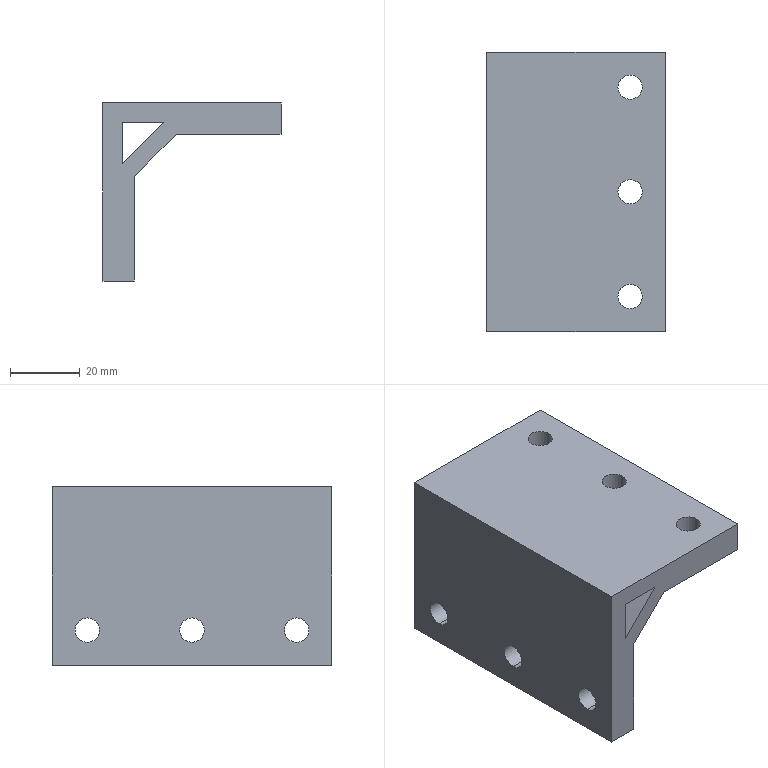Part | SolidWorks | features BaseBody 1 | 1 solid | 24 faces | box 51 x 80 x 51 mm | volume 64882 mm3 | cylinder 12 | plane 12 | commonest cylinder face diameters 7 x12
STEP:
#1=CARTESIAN_POINT('',(44.5,-30.,0.));
#2=VERTEX_POINT('',#1);
#3=CARTESIAN_POINT('',(37.5,-30.,0.));
#4=VERTEX_POINT('',#3);
#5=CARTESIAN_POINT('',(41.,-30.,0.));
#6=DIRECTION('',(0.,0.,-1.));
#7=DIRECTION('',(1.,0.,0.));
#8=AXIS2_PLACEMENT_3D('',#5,#6,#7);
#9=CIRCLE('',#8,3.5);
#10=EDGE_CURVE('',#2,#4,#9,.T.);
#11=ORIENTED_EDGE('',*,*,#10,.F.);
#12=CARTESIAN_POINT('',(44.5,-30.,-9.));
#13=VERTEX_POINT('',#12);
#14=CARTESIAN_POINT('',(44.5,-30.,0.));
#15=DIRECTION('',(0.,0.,-1.));
#16=VECTOR('',#15,1000.);
#17=LINE('',#14,#16);
#18=EDGE_CURVE('',#2,#13,#17,.T.);
#19=ORIENTED_EDGE('',*,*,#18,.T.);
#20=CARTESIAN_POINT('',(37.5,-30.,-9.));
#21=VERTEX_POINT('',#20);
#22=CARTESIAN_POINT('',(41.,-30.,-9.));
#23=DIRECTION('',(0.,0.,-1.));
#24=DIRECTION('',(1.,0.,0.));
#25=AXIS2_PLACEMENT_3D('',#22,#23,#24);
#26=CIRCLE('',#25,3.5);
#27=EDGE_CURVE('',#13,#21,#26,.T.);
#28=ORIENTED_EDGE('',*,*,#27,.T.);
#29=CARTESIAN_POINT('',(37.5,-30.,0.));
#30=DIRECTION('',(0.,0.,-1.));
#31=VECTOR('',#30,1000.);
#32=LINE('',#29,#31);
#33=EDGE_CURVE('',#4,#21,#32,.T.);
#34=ORIENTED_EDGE('',*,*,#33,.F.);
#35=EDGE_LOOP('',(#11,#19,#28,#34));
#36=FACE_OUTER_BOUND('',#35,.T.);
#37=CARTESIAN_POINT('',(41.,-30.,0.));
#38=DIRECTION('',(0.,0.,-1.));
#39=DIRECTION('',(-1.,0.,0.));
#40=AXIS2_PLACEMENT_3D('',#37,#38,#39);
#41=CYLINDRICAL_SURFACE('',#40,3.5);
#42=ADVANCED_FACE('',(#36),#41,.F.);
#43=CARTESIAN_POINT('',(44.5,0.,0.));
#44=VERTEX_POINT('',#43);
#45=CARTESIAN_POINT('',(37.5,0.,0.));
#46=VERTEX_POINT('',#45);
#47=CARTESIAN_POINT('',(41.,0.,0.));
#48=DIRECTION('',(0.,0.,-1.));
#49=DIRECTION('',(-1.,0.,0.));
#50=AXIS2_PLACEMENT_3D('',#47,#48,#49);
#51=CIRCLE('',#50,3.5);
#52=EDGE_CURVE('',#44,#46,#51,.T.);
#53=ORIENTED_EDGE('',*,*,#52,.F.);
#54=CARTESIAN_POINT('',(44.5,0.,-9.));
#55=VERTEX_POINT('',#54);
#56=CARTESIAN_POINT('',(44.5,0.,0.));
#57=DIRECTION('',(0.,0.,-1.));
#58=VECTOR('',#57,1000.);
#59=LINE('',#56,#58);
#60=EDGE_CURVE('',#44,#55,#59,.T.);
#61=ORIENTED_EDGE('',*,*,#60,.T.);
#62=CARTESIAN_POINT('',(37.5,0.,-9.));
#63=VERTEX_POINT('',#62);
#64=CARTESIAN_POINT('',(41.,0.,-9.));
#65=DIRECTION('',(0.,0.,-1.));
#66=DIRECTION('',(-1.,0.,0.));
#67=AXIS2_PLACEMENT_3D('',#64,#65,#66);
#68=CIRCLE('',#67,3.5);
#69=EDGE_CURVE('',#55,#63,#68,.T.);
#70=ORIENTED_EDGE('',*,*,#69,.T.);
#71=CARTESIAN_POINT('',(37.5,0.,0.));
#72=DIRECTION('',(0.,0.,-1.));
#73=VECTOR('',#72,1000.);
#74=LINE('',#71,#73);
#75=EDGE_CURVE('',#46,#63,#74,.T.);
#76=ORIENTED_EDGE('',*,*,#75,.F.);
#77=EDGE_LOOP('',(#53,#61,#70,#76));
#78=FACE_OUTER_BOUND('',#77,.T.);
#79=CARTESIAN_POINT('',(41.,0.,0.));
#80=DIRECTION('',(0.,0.,-1.));
#81=DIRECTION('',(-1.,0.,0.));
#82=AXIS2_PLACEMENT_3D('',#79,#80,#81);
#83=CYLINDRICAL_SURFACE('',#82,3.5);
#84=ADVANCED_FACE('',(#78),#83,.F.);
#85=CARTESIAN_POINT('',(44.5,30.,0.));
#86=VERTEX_POINT('',#85);
#87=CARTESIAN_POINT('',(37.5,30.,0.));
#88=VERTEX_POINT('',#87);
#89=CARTESIAN_POINT('',(41.,30.,0.));
#90=DIRECTION('',(0.,0.,-1.));
#91=DIRECTION('',(-1.,0.,0.));
#92=AXIS2_PLACEMENT_3D('',#89,#90,#91);
#93=CIRCLE('',#92,3.5);
#94=EDGE_CURVE('',#86,#88,#93,.T.);
#95=ORIENTED_EDGE('',*,*,#94,.F.);
#96=CARTESIAN_POINT('',(44.5,30.,-9.));
#97=VERTEX_POINT('',#96);
#98=CARTESIAN_POINT('',(44.5,30.,0.));
#99=DIRECTION('',(0.,0.,-1.));
#100=VECTOR('',#99,1000.);
#101=LINE('',#98,#100);
#102=EDGE_CURVE('',#86,#97,#101,.T.);
#103=ORIENTED_EDGE('',*,*,#102,.T.);
#104=CARTESIAN_POINT('',(37.5,30.,-9.));
#105=VERTEX_POINT('',#104);
#106=CARTESIAN_POINT('',(41.,30.,-9.));
#107=DIRECTION('',(0.,0.,-1.));
#108=DIRECTION('',(-1.,0.,0.));
#109=AXIS2_PLACEMENT_3D('',#106,#107,#108);
#110=CIRCLE('',#109,3.5);
#111=EDGE_CURVE('',#97,#105,#110,.T.);
#112=ORIENTED_EDGE('',*,*,#111,.T.);
#113=CARTESIAN_POINT('',(37.5,30.,0.));
#114=DIRECTION('',(0.,0.,-1.));
#115=VECTOR('',#114,1000.);
#116=LINE('',#113,#115);
#117=EDGE_CURVE('',#88,#105,#116,.T.);
#118=ORIENTED_EDGE('',*,*,#117,.F.);
#119=EDGE_LOOP('',(#95,#103,#112,#118));
#120=FACE_OUTER_BOUND('',#119,.T.);
#121=CARTESIAN_POINT('',(41.,30.,0.));
#122=DIRECTION('',(0.,0.,-1.));
#123=DIRECTION('',(-1.,0.,0.));
#124=AXIS2_PLACEMENT_3D('',#121,#122,#123);
#125=CYLINDRICAL_SURFACE('',#124,3.5);
#126=ADVANCED_FACE('',(#120),#125,.F.);
#127=CARTESIAN_POINT('',(0.,-30.,-37.5));
#128=VERTEX_POINT('',#127);
#129=CARTESIAN_POINT('',(0.,-30.,-44.5));
#130=VERTEX_POINT('',#129);
#131=CARTESIAN_POINT('',(0.,-30.,-41.));
#132=DIRECTION('',(1.,0.,0.));
#133=DIRECTION('',(0.,0.,1.));
#134=AXIS2_PLACEMENT_3D('',#131,#132,#133);
#135=CIRCLE('',#134,3.5);
#136=EDGE_CURVE('',#128,#130,#135,.T.);
#137=ORIENTED_EDGE('',*,*,#136,.F.);
#138=CARTESIAN_POINT('',(9.,-30.,-37.5));
#139=VERTEX_POINT('',#138);
#140=CARTESIAN_POINT('',(0.,-30.,-37.5));
#141=DIRECTION('',(1.,0.,0.));
#142=VECTOR('',#141,1000.);
#143=LINE('',#140,#142);
#144=EDGE_CURVE('',#128,#139,#143,.T.);
#145=ORIENTED_EDGE('',*,*,#144,.T.);
#146=CARTESIAN_POINT('',(9.,-30.,-44.5));
#147=VERTEX_POINT('',#146);
#148=CARTESIAN_POINT('',(9.,-30.,-41.));
#149=DIRECTION('',(1.,0.,0.));
#150=DIRECTION('',(0.,0.,1.));
#151=AXIS2_PLACEMENT_3D('',#148,#149,#150);
#152=CIRCLE('',#151,3.5);
#153=EDGE_CURVE('',#139,#147,#152,.T.);
#154=ORIENTED_EDGE('',*,*,#153,.T.);
#155=CARTESIAN_POINT('',(0.,-30.,-44.5));
#156=DIRECTION('',(1.,0.,0.));
#157=VECTOR('',#156,1000.);
#158=LINE('',#155,#157);
#159=EDGE_CURVE('',#130,#147,#158,.T.);
#160=ORIENTED_EDGE('',*,*,#159,.F.);
#161=EDGE_LOOP('',(#137,#145,#154,#160));
#162=FACE_OUTER_BOUND('',#161,.T.);
#163=CARTESIAN_POINT('',(0.,-30.,-41.));
#164=DIRECTION('',(1.,0.,0.));
#165=DIRECTION('',(0.,0.,-1.));
#166=AXIS2_PLACEMENT_3D('',#163,#164,#165);
#167=CYLINDRICAL_SURFACE('',#166,3.5);
#168=ADVANCED_FACE('',(#162),#167,.F.);
#169=CARTESIAN_POINT('',(0.,30.,-37.5));
#170=VERTEX_POINT('',#169);
#171=CARTESIAN_POINT('',(0.,30.,-44.5));
#172=VERTEX_POINT('',#171);
#173=CARTESIAN_POINT('',(0.,30.,-41.));
#174=DIRECTION('',(1.,0.,0.));
#175=DIRECTION('',(0.,0.,-1.));
#176=AXIS2_PLACEMENT_3D('',#173,#174,#175);
#177=CIRCLE('',#176,3.5);
#178=EDGE_CURVE('',#170,#172,#177,.T.);
#179=ORIENTED_EDGE('',*,*,#178,.F.);
#180=CARTESIAN_POINT('',(9.,30.,-37.5));
#181=VERTEX_POINT('',#180);
#182=CARTESIAN_POINT('',(0.,30.,-37.5));
#183=DIRECTION('',(1.,0.,0.));
#184=VECTOR('',#183,1000.);
#185=LINE('',#182,#184);
#186=EDGE_CURVE('',#170,#181,#185,.T.);
#187=ORIENTED_EDGE('',*,*,#186,.T.);
#188=CARTESIAN_POINT('',(9.,30.,-44.5));
#189=VERTEX_POINT('',#188);
#190=CARTESIAN_POINT('',(9.,30.,-41.));
#191=DIRECTION('',(1.,0.,0.));
#192=DIRECTION('',(0.,0.,-1.));
#193=AXIS2_PLACEMENT_3D('',#190,#191,#192);
#194=CIRCLE('',#193,3.5);
#195=EDGE_CURVE('',#181,#189,#194,.T.);
#196=ORIENTED_EDGE('',*,*,#195,.T.);
#197=CARTESIAN_POINT('',(0.,30.,-44.5));
#198=DIRECTION('',(1.,0.,0.));
#199=VECTOR('',#198,1000.);
#200=LINE('',#197,#199);
#201=EDGE_CURVE('',#172,#189,#200,.T.);
#202=ORIENTED_EDGE('',*,*,#201,.F.);
#203=EDGE_LOOP('',(#179,#187,#196,#202));
#204=FACE_OUTER_BOUND('',#203,.T.);
#205=CARTESIAN_POINT('',(0.,30.,-41.));
#206=DIRECTION('',(1.,0.,0.));
#207=DIRECTION('',(0.,0.,-1.));
#208=AXIS2_PLACEMENT_3D('',#205,#206,#207);
#209=CYLINDRICAL_SURFACE('',#208,3.5);
#210=ADVANCED_FACE('',(#204),#209,.F.);
#211=CARTESIAN_POINT('',(0.,0.,-37.5));
#212=VERTEX_POINT('',#211);
#213=CARTESIAN_POINT('',(0.,0.,-44.5));
#214=VERTEX_POINT('',#213);
#215=CARTESIAN_POINT('',(0.,0.,-41.));
#216=DIRECTION('',(1.,0.,0.));
#217=DIRECTION('',(0.,0.,-1.));
#218=AXIS2_PLACEMENT_3D('',#215,#216,#217);
#219=CIRCLE('',#218,3.5);
#220=EDGE_CURVE('',#212,#214,#219,.T.);
#221=ORIENTED_EDGE('',*,*,#220,.F.);
#222=CARTESIAN_POINT('',(9.,0.,-37.5));
#223=VERTEX_POINT('',#222);
#224=CARTESIAN_POINT('',(0.,0.,-37.5));
#225=DIRECTION('',(1.,0.,0.));
#226=VECTOR('',#225,1000.);
#227=LINE('',#224,#226);
#228=EDGE_CURVE('',#212,#223,#227,.T.);
#229=ORIENTED_EDGE('',*,*,#228,.T.);
#230=CARTESIAN_POINT('',(9.,0.,-44.5));
#231=VERTEX_POINT('',#230);
#232=CARTESIAN_POINT('',(9.,0.,-41.));
#233=DIRECTION('',(1.,0.,0.));
#234=DIRECTION('',(0.,0.,-1.));
#235=AXIS2_PLACEMENT_3D('',#232,#233,#234);
#236=CIRCLE('',#235,3.5);
#237=EDGE_CURVE('',#223,#231,#236,.T.);
#238=ORIENTED_EDGE('',*,*,#237,.T.);
#239=CARTESIAN_POINT('',(0.,0.,-44.5));
#240=DIRECTION('',(1.,0.,0.));
#241=VECTOR('',#240,1000.);
#242=LINE('',#239,#241);
#243=EDGE_CURVE('',#214,#231,#242,.T.);
#244=ORIENTED_EDGE('',*,*,#243,.F.);
#245=EDGE_LOOP('',(#221,#229,#238,#244));
#246=FACE_OUTER_BOUND('',#245,.T.);
#247=CARTESIAN_POINT('',(0.,0.,-41.));
#248=DIRECTION('',(1.,0.,0.));
#249=DIRECTION('',(0.,0.,-1.));
#250=AXIS2_PLACEMENT_3D('',#247,#248,#249);
#251=CYLINDRICAL_SURFACE('',#250,3.5);
#252=ADVANCED_FACE('',(#246),#251,.F.);
#253=CARTESIAN_POINT('',(17.464,40.,-5.464));
#254=VERTEX_POINT('',#253);
#255=CARTESIAN_POINT('',(5.464,40.,-17.464));
#256=VERTEX_POINT('',#255);
#257=CARTESIAN_POINT('',(17.464,40.,-5.464));
#258=DIRECTION('',(-0.7071,0.,-0.7071));
#259=VECTOR('',#258,1000.);
#260=LINE('',#257,#259);
#261=EDGE_CURVE('',#254,#256,#260,.T.);
#262=ORIENTED_EDGE('',*,*,#261,.T.);
#263=CARTESIAN_POINT('',(5.464,-40.,-17.464));
#264=VERTEX_POINT('',#263);
#265=CARTESIAN_POINT('',(5.464,-40.,-17.464));
#266=DIRECTION('',(0.,1.,0.));
#267=VECTOR('',#266,1000.);
#268=LINE('',#265,#267);
#269=EDGE_CURVE('',#264,#256,#268,.T.);
#270=ORIENTED_EDGE('',*,*,#269,.F.);
#271=CARTESIAN_POINT('',(17.464,-40.,-5.464));
#272=VERTEX_POINT('',#271);
#273=CARTESIAN_POINT('',(17.464,-40.,-5.464));
#274=DIRECTION('',(-0.7071,0.,-0.7071));
#275=VECTOR('',#274,1000.);
#276=LINE('',#273,#275);
#277=EDGE_CURVE('',#272,#264,#276,.T.);
#278=ORIENTED_EDGE('',*,*,#277,.F.);
#279=CARTESIAN_POINT('',(17.464,-40.,-5.464));
#280=DIRECTION('',(0.,1.,0.));
#281=VECTOR('',#280,1000.);
#282=LINE('',#279,#281);
#283=EDGE_CURVE('',#272,#254,#282,.T.);
#284=ORIENTED_EDGE('',*,*,#283,.T.);
#285=EDGE_LOOP('',(#262,#270,#278,#284));
#286=FACE_OUTER_BOUND('',#285,.T.);
#287=CARTESIAN_POINT('',(17.464,-40.,-5.464));
#288=DIRECTION('',(0.7071,0.,-0.7071));
#289=DIRECTION('',(0.,-1.,0.));
#290=AXIS2_PLACEMENT_3D('',#287,#288,#289);
#291=PLANE('',#290);
#292=ADVANCED_FACE('',(#286),#291,.F.);
#293=CARTESIAN_POINT('',(5.464,40.,-5.464));
#294=VERTEX_POINT('',#293);
#295=CARTESIAN_POINT('',(5.464,40.,-17.464));
#296=DIRECTION('',(0.,0.,1.));
#297=VECTOR('',#296,1000.);
#298=LINE('',#295,#297);
#299=EDGE_CURVE('',#256,#294,#298,.T.);
#300=ORIENTED_EDGE('',*,*,#299,.T.);
#301=CARTESIAN_POINT('',(5.464,-40.,-5.464));
#302=VERTEX_POINT('',#301);
#303=CARTESIAN_POINT('',(5.464,-40.,-5.464));
#304=DIRECTION('',(0.,1.,0.));
#305=VECTOR('',#304,1000.);
#306=LINE('',#303,#305);
#307=EDGE_CURVE('',#302,#294,#306,.T.);
#308=ORIENTED_EDGE('',*,*,#307,.F.);
#309=CARTESIAN_POINT('',(5.464,-40.,-17.464));
#310=DIRECTION('',(0.,0.,1.));
#311=VECTOR('',#310,1000.);
#312=LINE('',#309,#311);
#313=EDGE_CURVE('',#264,#302,#312,.T.);
#314=ORIENTED_EDGE('',*,*,#313,.F.);
#315=ORIENTED_EDGE('',*,*,#269,.T.);
#316=EDGE_LOOP('',(#300,#308,#314,#315));
#317=FACE_OUTER_BOUND('',#316,.T.);
#318=CARTESIAN_POINT('',(5.464,-40.,-17.464));
#319=DIRECTION('',(-1.,0.,0.));
#320=DIRECTION('',(0.,0.,1.));
#321=AXIS2_PLACEMENT_3D('',#318,#319,#320);
#322=PLANE('',#321);
#323=ADVANCED_FACE('',(#317),#322,.F.);
#324=CARTESIAN_POINT('',(5.464,40.,-5.464));
#325=DIRECTION('',(1.,0.,0.));
#326=VECTOR('',#325,1000.);
#327=LINE('',#324,#326);
#328=EDGE_CURVE('',#294,#254,#327,.T.);
#329=ORIENTED_EDGE('',*,*,#328,.T.);
#330=ORIENTED_EDGE('',*,*,#283,.F.);
#331=CARTESIAN_POINT('',(5.464,-40.,-5.464));
#332=DIRECTION('',(1.,0.,0.));
#333=VECTOR('',#332,1000.);
#334=LINE('',#331,#333);
#335=EDGE_CURVE('',#302,#272,#334,.T.);
#336=ORIENTED_EDGE('',*,*,#335,.F.);
#337=ORIENTED_EDGE('',*,*,#307,.T.);
#338=EDGE_LOOP('',(#329,#330,#336,#337));
#339=FACE_OUTER_BOUND('',#338,.T.);
#340=CARTESIAN_POINT('',(5.464,-40.,-5.464));
#341=DIRECTION('',(0.,0.,1.));
#342=DIRECTION('',(1.,0.,0.));
#343=AXIS2_PLACEMENT_3D('',#340,#341,#342);
#344=PLANE('',#343);
#345=ADVANCED_FACE('',(#339),#344,.F.);
#346=ORIENTED_EDGE('',*,*,#313,.T.);
#347=ORIENTED_EDGE('',*,*,#335,.T.);
#348=ORIENTED_EDGE('',*,*,#277,.T.);
#349=EDGE_LOOP('',(#346,#347,#348));
#350=FACE_BOUND('',#349,.T.);
#351=CARTESIAN_POINT('',(9.,-40.,-51.));
#352=VERTEX_POINT('',#351);
#353=CARTESIAN_POINT('',(0.,-40.,-51.));
#354=VERTEX_POINT('',#353);
#355=CARTESIAN_POINT('',(9.,-40.,-51.));
#356=DIRECTION('',(-1.,0.,0.));
#357=VECTOR('',#356,1000.);
#358=LINE('',#355,#357);
#359=EDGE_CURVE('',#352,#354,#358,.T.);
#360=ORIENTED_EDGE('',*,*,#359,.F.);
#361=CARTESIAN_POINT('',(9.,-40.,-21.));
#362=VERTEX_POINT('',#361);
#363=CARTESIAN_POINT('',(9.,-40.,-21.));
#364=DIRECTION('',(0.,0.,-1.));
#365=VECTOR('',#364,1000.);
#366=LINE('',#363,#365);
#367=EDGE_CURVE('',#362,#352,#366,.T.);
#368=ORIENTED_EDGE('',*,*,#367,.F.);
#369=CARTESIAN_POINT('',(21.,-40.,-9.));
#370=VERTEX_POINT('',#369);
#371=CARTESIAN_POINT('',(21.,-40.,-9.));
#372=DIRECTION('',(-0.7071,0.,-0.7071));
#373=VECTOR('',#372,1000.);
#374=LINE('',#371,#373);
#375=EDGE_CURVE('',#370,#362,#374,.T.);
#376=ORIENTED_EDGE('',*,*,#375,.F.);
#377=CARTESIAN_POINT('',(51.,-40.,-9.));
#378=VERTEX_POINT('',#377);
#379=CARTESIAN_POINT('',(51.,-40.,-9.));
#380=DIRECTION('',(-1.,0.,0.));
#381=VECTOR('',#380,1000.);
#382=LINE('',#379,#381);
#383=EDGE_CURVE('',#378,#370,#382,.T.);
#384=ORIENTED_EDGE('',*,*,#383,.F.);
#385=CARTESIAN_POINT('',(51.,-40.,0.));
#386=VERTEX_POINT('',#385);
#387=CARTESIAN_POINT('',(51.,-40.,0.));
#388=DIRECTION('',(0.,0.,-1.));
#389=VECTOR('',#388,1000.);
#390=LINE('',#387,#389);
#391=EDGE_CURVE('',#386,#378,#390,.T.);
#392=ORIENTED_EDGE('',*,*,#391,.F.);
#393=CARTESIAN_POINT('',(0.,-40.,0.));
#394=VERTEX_POINT('',#393);
#395=CARTESIAN_POINT('',(0.,-40.,0.));
#396=DIRECTION('',(1.,0.,0.));
#397=VECTOR('',#396,1000.);
#398=LINE('',#395,#397);
#399=EDGE_CURVE('',#394,#386,#398,.T.);
#400=ORIENTED_EDGE('',*,*,#399,.F.);
#401=CARTESIAN_POINT('',(0.,-40.,-51.));
#402=DIRECTION('',(0.,0.,1.));
#403=VECTOR('',#402,1000.);
#404=LINE('',#401,#403);
#405=EDGE_CURVE('',#354,#394,#404,.T.);
#406=ORIENTED_EDGE('',*,*,#405,.F.);
#407=EDGE_LOOP('',(#360,#368,#376,#384,#392,#400,#406));
#408=FACE_OUTER_BOUND('',#407,.T.);
#409=CARTESIAN_POINT('',(0.,-40.,0.));
#410=DIRECTION('',(0.,1.,0.));
#411=DIRECTION('',(1.,0.,0.));
#412=AXIS2_PLACEMENT_3D('',#409,#410,#411);
#413=PLANE('',#412);
#414=ADVANCED_FACE('',(#350,#408),#413,.F.);
#415=ORIENTED_EDGE('',*,*,#328,.F.);
#416=ORIENTED_EDGE('',*,*,#299,.F.);
#417=ORIENTED_EDGE('',*,*,#261,.F.);
#418=EDGE_LOOP('',(#415,#416,#417));
#419=FACE_BOUND('',#418,.T.);
#420=CARTESIAN_POINT('',(9.,40.,-51.));
#421=VERTEX_POINT('',#420);
#422=CARTESIAN_POINT('',(0.,40.,-51.));
#423=VERTEX_POINT('',#422);
#424=CARTESIAN_POINT('',(9.,40.,-51.));
#425=DIRECTION('',(-1.,0.,0.));
#426=VECTOR('',#425,1000.);
#427=LINE('',#424,#426);
#428=EDGE_CURVE('',#421,#423,#427,.T.);
#429=ORIENTED_EDGE('',*,*,#428,.T.);
#430=CARTESIAN_POINT('',(0.,40.,0.));
#431=VERTEX_POINT('',#430);
#432=CARTESIAN_POINT('',(0.,40.,-51.));
#433=DIRECTION('',(0.,0.,1.));
#434=VECTOR('',#433,1000.);
#435=LINE('',#432,#434);
#436=EDGE_CURVE('',#423,#431,#435,.T.);
#437=ORIENTED_EDGE('',*,*,#436,.T.);
#438=CARTESIAN_POINT('',(51.,40.,0.));
#439=VERTEX_POINT('',#438);
#440=CARTESIAN_POINT('',(0.,40.,0.));
#441=DIRECTION('',(1.,0.,0.));
#442=VECTOR('',#441,1000.);
#443=LINE('',#440,#442);
#444=EDGE_CURVE('',#431,#439,#443,.T.);
#445=ORIENTED_EDGE('',*,*,#444,.T.);
#446=CARTESIAN_POINT('',(51.,40.,-9.));
#447=VERTEX_POINT('',#446);
#448=CARTESIAN_POINT('',(51.,40.,0.));
#449=DIRECTION('',(0.,0.,-1.));
#450=VECTOR('',#449,1000.);
#451=LINE('',#448,#450);
#452=EDGE_CURVE('',#439,#447,#451,.T.);
#453=ORIENTED_EDGE('',*,*,#452,.T.);
#454=CARTESIAN_POINT('',(21.,40.,-9.));
#455=VERTEX_POINT('',#454);
#456=CARTESIAN_POINT('',(51.,40.,-9.));
#457=DIRECTION('',(-1.,0.,0.));
#458=VECTOR('',#457,1000.);
#459=LINE('',#456,#458);
#460=EDGE_CURVE('',#447,#455,#459,.T.);
#461=ORIENTED_EDGE('',*,*,#460,.T.);
#462=CARTESIAN_POINT('',(9.,40.,-21.));
#463=VERTEX_POINT('',#462);
#464=CARTESIAN_POINT('',(21.,40.,-9.));
#465=DIRECTION('',(-0.7071,0.,-0.7071));
#466=VECTOR('',#465,1000.);
#467=LINE('',#464,#466);
#468=EDGE_CURVE('',#455,#463,#467,.T.);
#469=ORIENTED_EDGE('',*,*,#468,.T.);
#470=CARTESIAN_POINT('',(9.,40.,-21.));
#471=DIRECTION('',(0.,0.,-1.));
#472=VECTOR('',#471,1000.);
#473=LINE('',#470,#472);
#474=EDGE_CURVE('',#463,#421,#473,.T.);
#475=ORIENTED_EDGE('',*,*,#474,.T.);
#476=EDGE_LOOP('',(#429,#437,#445,#453,#461,#469,#475));
#477=FACE_OUTER_BOUND('',#476,.T.);
#478=CARTESIAN_POINT('',(0.,40.,0.));
#479=DIRECTION('',(0.,1.,0.));
#480=DIRECTION('',(1.,0.,0.));
#481=AXIS2_PLACEMENT_3D('',#478,#479,#480);
#482=PLANE('',#481);
#483=ADVANCED_FACE('',(#419,#477),#482,.T.);
#484=CARTESIAN_POINT('',(9.,0.,-41.));
#485=DIRECTION('',(1.,0.,0.));
#486=DIRECTION('',(0.,0.,-1.));
#487=AXIS2_PLACEMENT_3D('',#484,#485,#486);
#488=CIRCLE('',#487,3.5);
#489=EDGE_CURVE('',#231,#223,#488,.T.);
#490=ORIENTED_EDGE('',*,*,#489,.F.);
#491=ORIENTED_EDGE('',*,*,#237,.F.);
#492=EDGE_LOOP('',(#490,#491));
#493=FACE_BOUND('',#492,.T.);
#494=CARTESIAN_POINT('',(9.,30.,-41.));
#495=DIRECTION('',(1.,0.,0.));
#496=DIRECTION('',(0.,0.,-1.));
#497=AXIS2_PLACEMENT_3D('',#494,#495,#496);
#498=CIRCLE('',#497,3.5);
#499=EDGE_CURVE('',#189,#181,#498,.T.);
#500=ORIENTED_EDGE('',*,*,#499,.F.);
#501=ORIENTED_EDGE('',*,*,#195,.F.);
#502=EDGE_LOOP('',(#500,#501));
#503=FACE_BOUND('',#502,.T.);
#504=CARTESIAN_POINT('',(9.,-30.,-41.));
#505=DIRECTION('',(1.,0.,0.));
#506=DIRECTION('',(0.,0.,1.));
#507=AXIS2_PLACEMENT_3D('',#504,#505,#506);
#508=CIRCLE('',#507,3.5);
#509=EDGE_CURVE('',#147,#139,#508,.T.);
#510=ORIENTED_EDGE('',*,*,#509,.F.);
#511=ORIENTED_EDGE('',*,*,#153,.F.);
#512=EDGE_LOOP('',(#510,#511));
#513=FACE_BOUND('',#512,.T.);
#514=ORIENTED_EDGE('',*,*,#367,.T.);
#515=CARTESIAN_POINT('',(9.,40.,-51.));
#516=DIRECTION('',(0.,-1.,0.));
#517=VECTOR('',#516,1000.);
#518=LINE('',#515,#517);
#519=EDGE_CURVE('',#421,#352,#518,.T.);
#520=ORIENTED_EDGE('',*,*,#519,.F.);
#521=ORIENTED_EDGE('',*,*,#474,.F.);
#522=CARTESIAN_POINT('',(9.,40.,-21.));
#523=DIRECTION('',(0.,-1.,0.));
#524=VECTOR('',#523,1000.);
#525=LINE('',#522,#524);
#526=EDGE_CURVE('',#463,#362,#525,.T.);
#527=ORIENTED_EDGE('',*,*,#526,.T.);
#528=EDGE_LOOP('',(#514,#520,#521,#527));
#529=FACE_OUTER_BOUND('',#528,.T.);
#530=CARTESIAN_POINT('',(9.,40.,-21.));
#531=DIRECTION('',(-1.,0.,0.));
#532=DIRECTION('',(0.,0.,1.));
#533=AXIS2_PLACEMENT_3D('',#530,#531,#532);
#534=PLANE('',#533);
#535=ADVANCED_FACE('',(#493,#503,#513,#529),#534,.F.);
#536=ORIENTED_EDGE('',*,*,#375,.T.);
#537=ORIENTED_EDGE('',*,*,#526,.F.);
#538=ORIENTED_EDGE('',*,*,#468,.F.);
#539=CARTESIAN_POINT('',(21.,40.,-9.));
#540=DIRECTION('',(0.,-1.,0.));
#541=VECTOR('',#540,1000.);
#542=LINE('',#539,#541);
#543=EDGE_CURVE('',#455,#370,#542,.T.);
#544=ORIENTED_EDGE('',*,*,#543,.T.);
#545=EDGE_LOOP('',(#536,#537,#538,#544));
#546=FACE_OUTER_BOUND('',#545,.T.);
#547=CARTESIAN_POINT('',(21.,40.,-9.));
#548=DIRECTION('',(-0.7071,0.,0.7071));
#549=DIRECTION('',(0.,1.,0.));
#550=AXIS2_PLACEMENT_3D('',#547,#548,#549);
#551=PLANE('',#550);
#552=ADVANCED_FACE('',(#546),#551,.F.);
#553=CARTESIAN_POINT('',(41.,30.,-9.));
#554=DIRECTION('',(0.,0.,-1.));
#555=DIRECTION('',(-1.,0.,0.));
#556=AXIS2_PLACEMENT_3D('',#553,#554,#555);
#557=CIRCLE('',#556,3.5);
#558=EDGE_CURVE('',#105,#97,#557,.T.);
#559=ORIENTED_EDGE('',*,*,#558,.F.);
#560=ORIENTED_EDGE('',*,*,#111,.F.);
#561=EDGE_LOOP('',(#559,#560));
#562=FACE_BOUND('',#561,.T.);
#563=CARTESIAN_POINT('',(41.,0.,-9.));
#564=DIRECTION('',(0.,0.,-1.));
#565=DIRECTION('',(-1.,0.,0.));
#566=AXIS2_PLACEMENT_3D('',#563,#564,#565);
#567=CIRCLE('',#566,3.5);
#568=EDGE_CURVE('',#63,#55,#567,.T.);
#569=ORIENTED_EDGE('',*,*,#568,.F.);
#570=ORIENTED_EDGE('',*,*,#69,.F.);
#571=EDGE_LOOP('',(#569,#570));
#572=FACE_BOUND('',#571,.T.);
#573=CARTESIAN_POINT('',(41.,-30.,-9.));
#574=DIRECTION('',(0.,0.,-1.));
#575=DIRECTION('',(1.,0.,0.));
#576=AXIS2_PLACEMENT_3D('',#573,#574,#575);
#577=CIRCLE('',#576,3.5);
#578=EDGE_CURVE('',#21,#13,#577,.T.);
#579=ORIENTED_EDGE('',*,*,#578,.F.);
#580=ORIENTED_EDGE('',*,*,#27,.F.);
#581=EDGE_LOOP('',(#579,#580));
#582=FACE_BOUND('',#581,.T.);
#583=ORIENTED_EDGE('',*,*,#383,.T.);
#584=ORIENTED_EDGE('',*,*,#543,.F.);
#585=ORIENTED_EDGE('',*,*,#460,.F.);
#586=CARTESIAN_POINT('',(51.,40.,-9.));
#587=DIRECTION('',(0.,-1.,0.));
#588=VECTOR('',#587,1000.);
#589=LINE('',#586,#588);
#590=EDGE_CURVE('',#447,#378,#589,.T.);
#591=ORIENTED_EDGE('',*,*,#590,.T.);
#592=EDGE_LOOP('',(#583,#584,#585,#591));
#593=FACE_OUTER_BOUND('',#592,.T.);
#594=CARTESIAN_POINT('',(51.,40.,-9.));
#595=DIRECTION('',(0.,0.,1.));
#596=DIRECTION('',(1.,0.,0.));
#597=AXIS2_PLACEMENT_3D('',#594,#595,#596);
#598=PLANE('',#597);
#599=ADVANCED_FACE('',(#562,#572,#582,#593),#598,.F.);
#600=ORIENTED_EDGE('',*,*,#391,.T.);
#601=ORIENTED_EDGE('',*,*,#590,.F.);
#602=ORIENTED_EDGE('',*,*,#452,.F.);
#603=CARTESIAN_POINT('',(51.,40.,0.));
#604=DIRECTION('',(0.,-1.,0.));
#605=VECTOR('',#604,1000.);
#606=LINE('',#603,#605);
#607=EDGE_CURVE('',#439,#386,#606,.T.);
#608=ORIENTED_EDGE('',*,*,#607,.T.);
#609=EDGE_LOOP('',(#600,#601,#602,#608));
#610=FACE_OUTER_BOUND('',#609,.T.);
#611=CARTESIAN_POINT('',(51.,40.,0.));
#612=DIRECTION('',(-1.,0.,0.));
#613=DIRECTION('',(0.,0.,1.));
#614=AXIS2_PLACEMENT_3D('',#611,#612,#613);
#615=PLANE('',#614);
#616=ADVANCED_FACE('',(#610),#615,.F.);
#617=CARTESIAN_POINT('',(41.,30.,0.));
#618=DIRECTION('',(0.,0.,-1.));
#619=DIRECTION('',(-1.,0.,0.));
#620=AXIS2_PLACEMENT_3D('',#617,#618,#619);
#621=CIRCLE('',#620,3.5);
#622=EDGE_CURVE('',#88,#86,#621,.T.);
#623=ORIENTED_EDGE('',*,*,#622,.T.);
#624=ORIENTED_EDGE('',*,*,#94,.T.);
#625=EDGE_LOOP('',(#623,#624));
#626=FACE_BOUND('',#625,.T.);
#627=CARTESIAN_POINT('',(41.,0.,0.));
#628=DIRECTION('',(0.,0.,-1.));
#629=DIRECTION('',(-1.,0.,0.));
#630=AXIS2_PLACEMENT_3D('',#627,#628,#629);
#631=CIRCLE('',#630,3.5);
#632=EDGE_CURVE('',#46,#44,#631,.T.);
#633=ORIENTED_EDGE('',*,*,#632,.T.);
#634=ORIENTED_EDGE('',*,*,#52,.T.);
#635=EDGE_LOOP('',(#633,#634));
#636=FACE_BOUND('',#635,.T.);
#637=CARTESIAN_POINT('',(41.,-30.,0.));
#638=DIRECTION('',(0.,0.,-1.));
#639=DIRECTION('',(1.,0.,0.));
#640=AXIS2_PLACEMENT_3D('',#637,#638,#639);
#641=CIRCLE('',#640,3.5);
#642=EDGE_CURVE('',#4,#2,#641,.T.);
#643=ORIENTED_EDGE('',*,*,#642,.T.);
#644=ORIENTED_EDGE('',*,*,#10,.T.);
#645=EDGE_LOOP('',(#643,#644));
#646=FACE_BOUND('',#645,.T.);
#647=ORIENTED_EDGE('',*,*,#399,.T.);
#648=ORIENTED_EDGE('',*,*,#607,.F.);
#649=ORIENTED_EDGE('',*,*,#444,.F.);
#650=CARTESIAN_POINT('',(0.,40.,0.));
#651=DIRECTION('',(0.,-1.,0.));
#652=VECTOR('',#651,1000.);
#653=LINE('',#650,#652);
#654=EDGE_CURVE('',#431,#394,#653,.T.);
#655=ORIENTED_EDGE('',*,*,#654,.T.);
#656=EDGE_LOOP('',(#647,#648,#649,#655));
#657=FACE_OUTER_BOUND('',#656,.T.);
#658=CARTESIAN_POINT('',(0.,40.,0.));
#659=DIRECTION('',(0.,0.,-1.));
#660=DIRECTION('',(0.,-1.,0.));
#661=AXIS2_PLACEMENT_3D('',#658,#659,#660);
#662=PLANE('',#661);
#663=ADVANCED_FACE('',(#626,#636,#646,#657),#662,.F.);
#664=CARTESIAN_POINT('',(0.,0.,-41.));
#665=DIRECTION('',(1.,0.,0.));
#666=DIRECTION('',(0.,0.,-1.));
#667=AXIS2_PLACEMENT_3D('',#664,#665,#666);
#668=CIRCLE('',#667,3.5);
#669=EDGE_CURVE('',#214,#212,#668,.T.);
#670=ORIENTED_EDGE('',*,*,#669,.T.);
#671=ORIENTED_EDGE('',*,*,#220,.T.);
#672=EDGE_LOOP('',(#670,#671));
#673=FACE_BOUND('',#672,.T.);
#674=CARTESIAN_POINT('',(0.,30.,-41.));
#675=DIRECTION('',(1.,0.,0.));
#676=DIRECTION('',(0.,0.,-1.));
#677=AXIS2_PLACEMENT_3D('',#674,#675,#676);
#678=CIRCLE('',#677,3.5);
#679=EDGE_CURVE('',#172,#170,#678,.T.);
#680=ORIENTED_EDGE('',*,*,#679,.T.);
#681=ORIENTED_EDGE('',*,*,#178,.T.);
#682=EDGE_LOOP('',(#680,#681));
#683=FACE_BOUND('',#682,.T.);
#684=CARTESIAN_POINT('',(0.,-30.,-41.));
#685=DIRECTION('',(1.,0.,0.));
#686=DIRECTION('',(0.,0.,1.));
#687=AXIS2_PLACEMENT_3D('',#684,#685,#686);
#688=CIRCLE('',#687,3.5);
#689=EDGE_CURVE('',#130,#128,#688,.T.);
#690=ORIENTED_EDGE('',*,*,#689,.T.);
#691=ORIENTED_EDGE('',*,*,#136,.T.);
#692=EDGE_LOOP('',(#690,#691));
#693=FACE_BOUND('',#692,.T.);
#694=ORIENTED_EDGE('',*,*,#405,.T.);
#695=ORIENTED_EDGE('',*,*,#654,.F.);
#696=ORIENTED_EDGE('',*,*,#436,.F.);
#697=CARTESIAN_POINT('',(0.,40.,-51.));
#698=DIRECTION('',(0.,-1.,0.));
#699=VECTOR('',#698,1000.);
#700=LINE('',#697,#699);
#701=EDGE_CURVE('',#423,#354,#700,.T.);
#702=ORIENTED_EDGE('',*,*,#701,.T.);
#703=EDGE_LOOP('',(#694,#695,#696,#702));
#704=FACE_OUTER_BOUND('',#703,.T.);
#705=CARTESIAN_POINT('',(0.,40.,-51.));
#706=DIRECTION('',(1.,0.,0.));
#707=DIRECTION('',(0.,0.,1.));
#708=AXIS2_PLACEMENT_3D('',#705,#706,#707);
#709=PLANE('',#708);
#710=ADVANCED_FACE('',(#673,#683,#693,#704),#709,.F.);
#711=ORIENTED_EDGE('',*,*,#359,.T.);
#712=ORIENTED_EDGE('',*,*,#701,.F.);
#713=ORIENTED_EDGE('',*,*,#428,.F.);
#714=ORIENTED_EDGE('',*,*,#519,.T.);
#715=EDGE_LOOP('',(#711,#712,#713,#714));
#716=FACE_OUTER_BOUND('',#715,.T.);
#717=CARTESIAN_POINT('',(9.,40.,-51.));
#718=DIRECTION('',(0.,0.,1.));
#719=DIRECTION('',(1.,0.,0.));
#720=AXIS2_PLACEMENT_3D('',#717,#718,#719);
#721=PLANE('',#720);
#722=ADVANCED_FACE('',(#716),#721,.F.);
#723=ORIENTED_EDGE('',*,*,#228,.F.);
#724=ORIENTED_EDGE('',*,*,#669,.F.);
#725=ORIENTED_EDGE('',*,*,#243,.T.);
#726=ORIENTED_EDGE('',*,*,#489,.T.);
#727=EDGE_LOOP('',(#723,#724,#725,#726));
#728=FACE_OUTER_BOUND('',#727,.T.);
#729=CARTESIAN_POINT('',(0.,0.,-41.));
#730=DIRECTION('',(1.,0.,0.));
#731=DIRECTION('',(0.,0.,-1.));
#732=AXIS2_PLACEMENT_3D('',#729,#730,#731);
#733=CYLINDRICAL_SURFACE('',#732,3.5);
#734=ADVANCED_FACE('',(#728),#733,.F.);
#735=ORIENTED_EDGE('',*,*,#186,.F.);
#736=ORIENTED_EDGE('',*,*,#679,.F.);
#737=ORIENTED_EDGE('',*,*,#201,.T.);
#738=ORIENTED_EDGE('',*,*,#499,.T.);
#739=EDGE_LOOP('',(#735,#736,#737,#738));
#740=FACE_OUTER_BOUND('',#739,.T.);
#741=CARTESIAN_POINT('',(0.,30.,-41.));
#742=DIRECTION('',(1.,0.,0.));
#743=DIRECTION('',(0.,0.,-1.));
#744=AXIS2_PLACEMENT_3D('',#741,#742,#743);
#745=CYLINDRICAL_SURFACE('',#744,3.5);
#746=ADVANCED_FACE('',(#740),#745,.F.);
#747=ORIENTED_EDGE('',*,*,#144,.F.);
#748=ORIENTED_EDGE('',*,*,#689,.F.);
#749=ORIENTED_EDGE('',*,*,#159,.T.);
#750=ORIENTED_EDGE('',*,*,#509,.T.);
#751=EDGE_LOOP('',(#747,#748,#749,#750));
#752=FACE_OUTER_BOUND('',#751,.T.);
#753=CARTESIAN_POINT('',(0.,-30.,-41.));
#754=DIRECTION('',(1.,0.,0.));
#755=DIRECTION('',(0.,0.,-1.));
#756=AXIS2_PLACEMENT_3D('',#753,#754,#755);
#757=CYLINDRICAL_SURFACE('',#756,3.5);
#758=ADVANCED_FACE('',(#752),#757,.F.);
#759=ORIENTED_EDGE('',*,*,#102,.F.);
#760=ORIENTED_EDGE('',*,*,#622,.F.);
#761=ORIENTED_EDGE('',*,*,#117,.T.);
#762=ORIENTED_EDGE('',*,*,#558,.T.);
#763=EDGE_LOOP('',(#759,#760,#761,#762));
#764=FACE_OUTER_BOUND('',#763,.T.);
#765=CARTESIAN_POINT('',(41.,30.,0.));
#766=DIRECTION('',(0.,0.,-1.));
#767=DIRECTION('',(-1.,0.,0.));
#768=AXIS2_PLACEMENT_3D('',#765,#766,#767);
#769=CYLINDRICAL_SURFACE('',#768,3.5);
#770=ADVANCED_FACE('',(#764),#769,.F.);
#771=ORIENTED_EDGE('',*,*,#60,.F.);
#772=ORIENTED_EDGE('',*,*,#632,.F.);
#773=ORIENTED_EDGE('',*,*,#75,.T.);
#774=ORIENTED_EDGE('',*,*,#568,.T.);
#775=EDGE_LOOP('',(#771,#772,#773,#774));
#776=FACE_OUTER_BOUND('',#775,.T.);
#777=CARTESIAN_POINT('',(41.,0.,0.));
#778=DIRECTION('',(0.,0.,-1.));
#779=DIRECTION('',(-1.,0.,0.));
#780=AXIS2_PLACEMENT_3D('',#777,#778,#779);
#781=CYLINDRICAL_SURFACE('',#780,3.5);
#782=ADVANCED_FACE('',(#776),#781,.F.);
#783=ORIENTED_EDGE('',*,*,#18,.F.);
#784=ORIENTED_EDGE('',*,*,#642,.F.);
#785=ORIENTED_EDGE('',*,*,#33,.T.);
#786=ORIENTED_EDGE('',*,*,#578,.T.);
#787=EDGE_LOOP('',(#783,#784,#785,#786));
#788=FACE_OUTER_BOUND('',#787,.T.);
#789=CARTESIAN_POINT('',(41.,-30.,0.));
#790=DIRECTION('',(0.,0.,-1.));
#791=DIRECTION('',(-1.,0.,0.));
#792=AXIS2_PLACEMENT_3D('',#789,#790,#791);
#793=CYLINDRICAL_SURFACE('',#792,3.5);
#794=ADVANCED_FACE('',(#788),#793,.F.);
#795=CLOSED_SHELL('',(#42,#84,#126,#168,#210,#252,#292,#323,#345,#414,#483,#535,#552,#599,#616,#663,#710,#722,#734,#746,#758,#770,#782,#794));
#796=MANIFOLD_SOLID_BREP('',#795);
#797=CARTESIAN_POINT('',(0.,0.,0.));
#798=DIRECTION('',(0.,0.,1.));
#799=DIRECTION('',(1.,0.,0.));
#800=AXIS2_PLACEMENT_3D('',#797,#798,#799);
#801=(LENGTH_UNIT()NAMED_UNIT(*)SI_UNIT(.MILLI.,.METRE.));
#802=UNCERTAINTY_MEASURE_WITH_UNIT(LENGTH_MEASURE(0.00001),#801,'','');
#803=(NAMED_UNIT(*)PLANE_ANGLE_UNIT()SI_UNIT($,.RADIAN.));
#804=(NAMED_UNIT(*)SI_UNIT($,.STERADIAN.)SOLID_ANGLE_UNIT());
#805=(GEOMETRIC_REPRESENTATION_CONTEXT(3)GLOBAL_UNCERTAINTY_ASSIGNED_CONTEXT((#802))GLOBAL_UNIT_ASSIGNED_CONTEXT((#801,#803,#804))REPRESENTATION_CONTEXT('',''));
#806=ADVANCED_BREP_SHAPE_REPRESENTATION('',(#796,#800),#805);